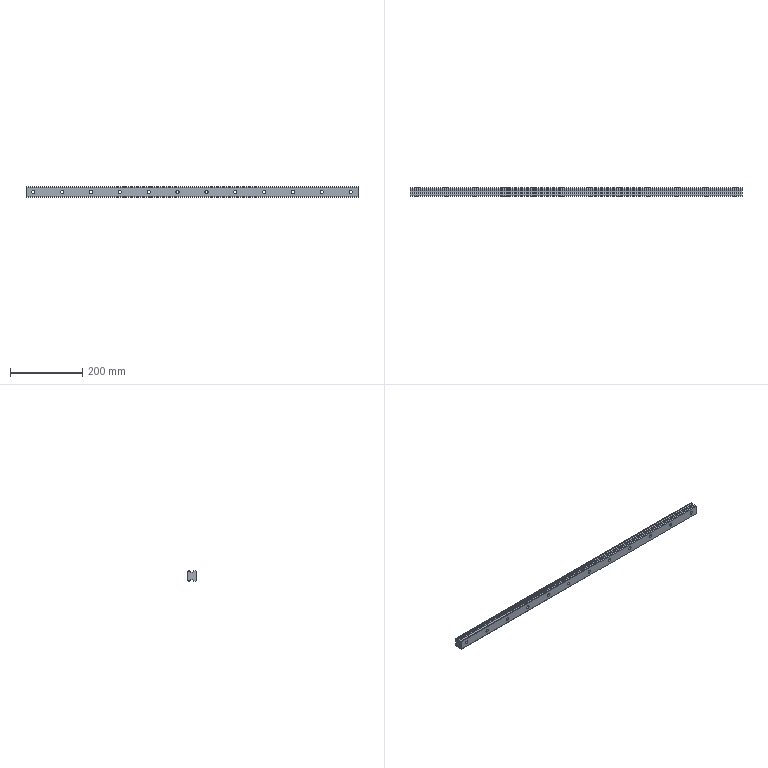Part | STEP file | J452-EBZ05-14-04-Part-3 | 1 solid | 97 faces | box 920 x 23 x 28 mm | volume 503072 mm3 | cylinder 69 | plane 28 | commonest cylinder face diameters 9 x24 14 x24 0.986 x3 0.995 x3 1.369 x3 0.952 x2